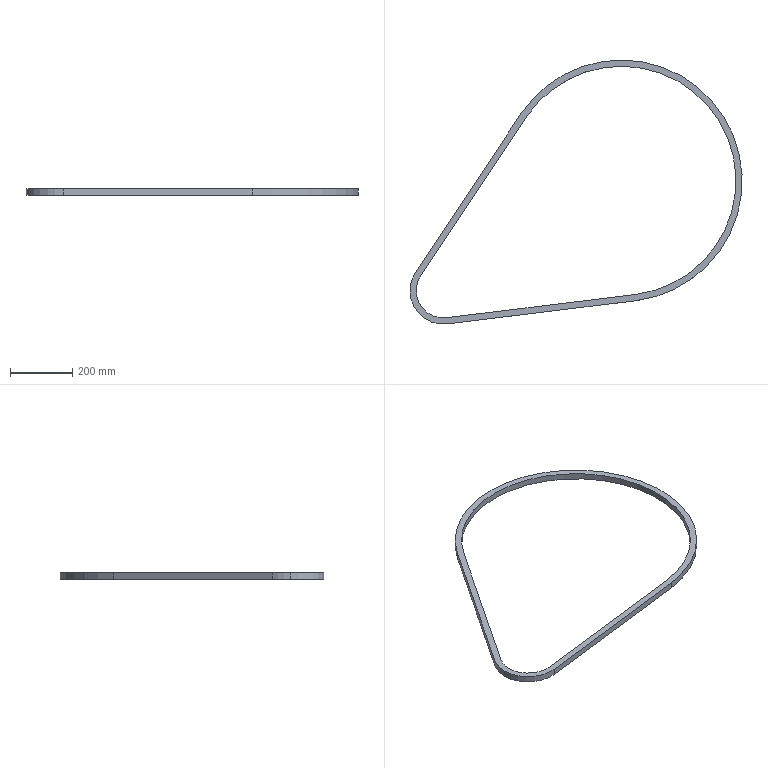Part | SolidWorks | features BaseBody 1 | 1 solid | 12 faces | box 1063 x 845.491 x 20 mm | volume 1178269 mm3 | cylinder 6 | plane 6 | commonest cylinder face diameters 173.589 x2 213.589 x2 733.102 x1 773.102 x1
STEP:
#1=CARTESIAN_POINT('',(-144.626,469.602,796.033));
#2=VERTEX_POINT('',#1);
#3=CARTESIAN_POINT('',(-513.842,1067.234,796.033));
#4=VERTEX_POINT('',#3);
#5=CARTESIAN_POINT('',(-191.923,853.249,796.033));
#6=DIRECTION('',(0.,0.,1.));
#7=DIRECTION('',(1.,0.,0.));
#8=AXIS2_PLACEMENT_3D('',#5,#6,#7);
#9=CIRCLE('',#8,386.551);
#10=EDGE_CURVE('',#2,#4,#9,.T.);
#11=ORIENTED_EDGE('',*,*,#10,.T.);
#12=CARTESIAN_POINT('',(-513.842,1067.234,816.033));
#13=VERTEX_POINT('',#12);
#14=CARTESIAN_POINT('',(-513.842,1067.234,816.033));
#15=DIRECTION('',(0.,0.,-1.));
#16=VECTOR('',#15,1000.);
#17=LINE('',#14,#16);
#18=EDGE_CURVE('',#13,#4,#17,.T.);
#19=ORIENTED_EDGE('',*,*,#18,.F.);
#20=CARTESIAN_POINT('',(-144.626,469.602,816.033));
#21=VERTEX_POINT('',#20);
#22=CARTESIAN_POINT('',(-191.923,853.249,816.033));
#23=DIRECTION('',(0.,0.,1.));
#24=DIRECTION('',(1.,0.,0.));
#25=AXIS2_PLACEMENT_3D('',#22,#23,#24);
#26=CIRCLE('',#25,386.551);
#27=EDGE_CURVE('',#21,#13,#26,.T.);
#28=ORIENTED_EDGE('',*,*,#27,.F.);
#29=CARTESIAN_POINT('',(-144.626,469.602,816.033));
#30=DIRECTION('',(0.,0.,-1.));
#31=VECTOR('',#30,1000.);
#32=LINE('',#29,#31);
#33=EDGE_CURVE('',#21,#2,#32,.T.);
#34=ORIENTED_EDGE('',*,*,#33,.T.);
#35=EDGE_LOOP('',(#11,#19,#28,#34));
#36=FACE_OUTER_BOUND('',#35,.T.);
#37=CARTESIAN_POINT('',(-191.923,853.249,816.033));
#38=DIRECTION('',(0.,0.,-1.));
#39=DIRECTION('',(-1.,0.,0.));
#40=AXIS2_PLACEMENT_3D('',#37,#38,#39);
#41=CYLINDRICAL_SURFACE('',#40,386.551);
#42=ADVANCED_FACE('',(#36),#41,.T.);
#43=CARTESIAN_POINT('',(-748.856,395.111,796.033));
#44=VERTEX_POINT('',#43);
#45=CARTESIAN_POINT('',(-748.856,395.111,796.033));
#46=DIRECTION('',(0.9925,0.1224,0.));
#47=VECTOR('',#46,1000.);
#48=LINE('',#45,#47);
#49=EDGE_CURVE('',#44,#2,#48,.T.);
#50=ORIENTED_EDGE('',*,*,#49,.T.);
#51=ORIENTED_EDGE('',*,*,#33,.F.);
#52=CARTESIAN_POINT('',(-748.856,395.111,816.033));
#53=VERTEX_POINT('',#52);
#54=CARTESIAN_POINT('',(-748.856,395.111,816.033));
#55=DIRECTION('',(0.9925,0.1224,0.));
#56=VECTOR('',#55,1000.);
#57=LINE('',#54,#56);
#58=EDGE_CURVE('',#53,#21,#57,.T.);
#59=ORIENTED_EDGE('',*,*,#58,.F.);
#60=CARTESIAN_POINT('',(-748.856,395.111,816.033));
#61=DIRECTION('',(0.,0.,-1.));
#62=VECTOR('',#61,1000.);
#63=LINE('',#60,#62);
#64=EDGE_CURVE('',#53,#44,#63,.T.);
#65=ORIENTED_EDGE('',*,*,#64,.T.);
#66=EDGE_LOOP('',(#50,#51,#59,#65));
#67=FACE_OUTER_BOUND('',#66,.T.);
#68=CARTESIAN_POINT('',(-748.856,395.111,816.033));
#69=DIRECTION('',(-0.1224,0.9925,0.));
#70=DIRECTION('',(0.,0.,1.));
#71=AXIS2_PLACEMENT_3D('',#68,#69,#70);
#72=PLANE('',#71);
#73=ADVANCED_FACE('',(#67),#72,.F.);
#74=CARTESIAN_POINT('',(-868.718,501.103,816.033));
#75=VERTEX_POINT('',#74);
#76=CARTESIAN_POINT('',(-868.718,501.103,796.033));
#77=VERTEX_POINT('',#76);
#78=CARTESIAN_POINT('',(-868.718,501.103,816.033));
#79=DIRECTION('',(0.,0.,-1.));
#80=VECTOR('',#79,1000.);
#81=LINE('',#78,#80);
#82=EDGE_CURVE('',#75,#77,#81,.T.);
#83=ORIENTED_EDGE('',*,*,#82,.F.);
#84=CARTESIAN_POINT('',(-850.862,560.222,816.033));
#85=VERTEX_POINT('',#84);
#86=CARTESIAN_POINT('',(-761.923,501.103,816.033));
#87=DIRECTION('',(0.,0.,1.));
#88=DIRECTION('',(1.,0.,0.));
#89=AXIS2_PLACEMENT_3D('',#86,#87,#88);
#90=CIRCLE('',#89,106.795);
#91=EDGE_CURVE('',#85,#75,#90,.T.);
#92=ORIENTED_EDGE('',*,*,#91,.F.);
#93=CARTESIAN_POINT('',(-850.862,560.222,796.033));
#94=VERTEX_POINT('',#93);
#95=CARTESIAN_POINT('',(-850.862,560.222,816.033));
#96=DIRECTION('',(0.,0.,-1.));
#97=VECTOR('',#96,1000.);
#98=LINE('',#95,#97);
#99=EDGE_CURVE('',#85,#94,#98,.T.);
#100=ORIENTED_EDGE('',*,*,#99,.T.);
#101=CARTESIAN_POINT('',(-761.923,501.103,796.033));
#102=DIRECTION('',(0.,0.,1.));
#103=DIRECTION('',(1.,0.,0.));
#104=AXIS2_PLACEMENT_3D('',#101,#102,#103);
#105=CIRCLE('',#104,106.795);
#106=EDGE_CURVE('',#94,#77,#105,.T.);
#107=ORIENTED_EDGE('',*,*,#106,.T.);
#108=EDGE_LOOP('',(#83,#92,#100,#107));
#109=FACE_OUTER_BOUND('',#108,.T.);
#110=CARTESIAN_POINT('',(-761.923,501.103,816.033));
#111=DIRECTION('',(0.,0.,-1.));
#112=DIRECTION('',(-1.,0.,0.));
#113=AXIS2_PLACEMENT_3D('',#110,#111,#112);
#114=CYLINDRICAL_SURFACE('',#113,106.795);
#115=ADVANCED_FACE('',(#109),#114,.T.);
#116=CARTESIAN_POINT('',(-513.842,1067.234,796.033));
#117=DIRECTION('',(-0.5536,-0.8328,0.));
#118=VECTOR('',#117,1000.);
#119=LINE('',#116,#118);
#120=EDGE_CURVE('',#4,#94,#119,.T.);
#121=ORIENTED_EDGE('',*,*,#120,.T.);
#122=ORIENTED_EDGE('',*,*,#99,.F.);
#123=CARTESIAN_POINT('',(-513.842,1067.234,816.033));
#124=DIRECTION('',(-0.5536,-0.8328,0.));
#125=VECTOR('',#124,1000.);
#126=LINE('',#123,#125);
#127=EDGE_CURVE('',#13,#85,#126,.T.);
#128=ORIENTED_EDGE('',*,*,#127,.F.);
#129=ORIENTED_EDGE('',*,*,#18,.T.);
#130=EDGE_LOOP('',(#121,#122,#128,#129));
#131=FACE_OUTER_BOUND('',#130,.T.);
#132=CARTESIAN_POINT('',(-513.842,1067.234,816.033));
#133=DIRECTION('',(0.8328,-0.5536,0.));
#134=DIRECTION('',(0.,0.,-1.));
#135=AXIS2_PLACEMENT_3D('',#132,#133,#134);
#136=PLANE('',#135);
#137=ADVANCED_FACE('',(#131),#136,.F.);
#138=CARTESIAN_POINT('',(-147.073,489.452,796.033));
#139=VERTEX_POINT('',#138);
#140=CARTESIAN_POINT('',(-497.186,1056.162,796.033));
#141=VERTEX_POINT('',#140);
#142=CARTESIAN_POINT('',(-191.923,853.249,796.033));
#143=DIRECTION('',(0.,0.,1.));
#144=DIRECTION('',(-1.,0.,0.));
#145=AXIS2_PLACEMENT_3D('',#142,#143,#144);
#146=CIRCLE('',#145,366.551);
#147=EDGE_CURVE('',#139,#141,#146,.T.);
#148=ORIENTED_EDGE('',*,*,#147,.F.);
#149=CARTESIAN_POINT('',(-147.073,489.452,816.033));
#150=VERTEX_POINT('',#149);
#151=CARTESIAN_POINT('',(-147.073,489.452,816.033));
#152=DIRECTION('',(0.,0.,-1.));
#153=VECTOR('',#152,1000.);
#154=LINE('',#151,#153);
#155=EDGE_CURVE('',#150,#139,#154,.T.);
#156=ORIENTED_EDGE('',*,*,#155,.F.);
#157=CARTESIAN_POINT('',(-497.186,1056.162,816.033));
#158=VERTEX_POINT('',#157);
#159=CARTESIAN_POINT('',(-191.923,853.249,816.033));
#160=DIRECTION('',(0.,0.,1.));
#161=DIRECTION('',(-1.,0.,0.));
#162=AXIS2_PLACEMENT_3D('',#159,#160,#161);
#163=CIRCLE('',#162,366.551);
#164=EDGE_CURVE('',#150,#158,#163,.T.);
#165=ORIENTED_EDGE('',*,*,#164,.T.);
#166=CARTESIAN_POINT('',(-497.186,1056.162,816.033));
#167=DIRECTION('',(0.,0.,-1.));
#168=VECTOR('',#167,1000.);
#169=LINE('',#166,#168);
#170=EDGE_CURVE('',#158,#141,#169,.T.);
#171=ORIENTED_EDGE('',*,*,#170,.T.);
#172=EDGE_LOOP('',(#148,#156,#165,#171));
#173=FACE_OUTER_BOUND('',#172,.T.);
#174=CARTESIAN_POINT('',(-191.923,853.249,816.033));
#175=DIRECTION('',(0.,0.,-1.));
#176=DIRECTION('',(-1.,0.,0.));
#177=AXIS2_PLACEMENT_3D('',#174,#175,#176);
#178=CYLINDRICAL_SURFACE('',#177,366.551);
#179=ADVANCED_FACE('',(#173),#178,.F.);
#180=CARTESIAN_POINT('',(-751.303,414.961,796.033));
#181=VERTEX_POINT('',#180);
#182=CARTESIAN_POINT('',(-751.303,414.961,796.033));
#183=DIRECTION('',(0.9925,0.1224,0.));
#184=VECTOR('',#183,1000.);
#185=LINE('',#182,#184);
#186=EDGE_CURVE('',#181,#139,#185,.T.);
#187=ORIENTED_EDGE('',*,*,#186,.F.);
#188=CARTESIAN_POINT('',(-751.303,414.961,816.033));
#189=VERTEX_POINT('',#188);
#190=CARTESIAN_POINT('',(-751.303,414.961,816.033));
#191=DIRECTION('',(0.,0.,-1.));
#192=VECTOR('',#191,1000.);
#193=LINE('',#190,#192);
#194=EDGE_CURVE('',#189,#181,#193,.T.);
#195=ORIENTED_EDGE('',*,*,#194,.F.);
#196=CARTESIAN_POINT('',(-751.303,414.961,816.033));
#197=DIRECTION('',(0.9925,0.1224,0.));
#198=VECTOR('',#197,1000.);
#199=LINE('',#196,#198);
#200=EDGE_CURVE('',#189,#150,#199,.T.);
#201=ORIENTED_EDGE('',*,*,#200,.T.);
#202=ORIENTED_EDGE('',*,*,#155,.T.);
#203=EDGE_LOOP('',(#187,#195,#201,#202));
#204=FACE_OUTER_BOUND('',#203,.T.);
#205=CARTESIAN_POINT('',(-751.303,414.961,816.033));
#206=DIRECTION('',(-0.1224,0.9925,0.));
#207=DIRECTION('',(0.,0.,1.));
#208=AXIS2_PLACEMENT_3D('',#205,#206,#207);
#209=PLANE('',#208);
#210=ADVANCED_FACE('',(#204),#209,.T.);
#211=CARTESIAN_POINT('',(-848.718,501.103,816.033));
#212=VERTEX_POINT('',#211);
#213=CARTESIAN_POINT('',(-848.718,501.103,796.033));
#214=VERTEX_POINT('',#213);
#215=CARTESIAN_POINT('',(-848.718,501.103,816.033));
#216=DIRECTION('',(0.,0.,-1.));
#217=VECTOR('',#216,1000.);
#218=LINE('',#215,#217);
#219=EDGE_CURVE('',#212,#214,#218,.T.);
#220=ORIENTED_EDGE('',*,*,#219,.F.);
#221=CARTESIAN_POINT('',(-761.923,501.103,816.033));
#222=DIRECTION('',(0.,0.,1.));
#223=DIRECTION('',(-1.,0.,0.));
#224=AXIS2_PLACEMENT_3D('',#221,#222,#223);
#225=CIRCLE('',#224,86.795);
#226=EDGE_CURVE('',#212,#189,#225,.T.);
#227=ORIENTED_EDGE('',*,*,#226,.T.);
#228=ORIENTED_EDGE('',*,*,#194,.T.);
#229=CARTESIAN_POINT('',(-761.923,501.103,796.033));
#230=DIRECTION('',(0.,0.,1.));
#231=DIRECTION('',(-1.,0.,0.));
#232=AXIS2_PLACEMENT_3D('',#229,#230,#231);
#233=CIRCLE('',#232,86.795);
#234=EDGE_CURVE('',#214,#181,#233,.T.);
#235=ORIENTED_EDGE('',*,*,#234,.F.);
#236=EDGE_LOOP('',(#220,#227,#228,#235));
#237=FACE_OUTER_BOUND('',#236,.T.);
#238=CARTESIAN_POINT('',(-761.923,501.103,816.033));
#239=DIRECTION('',(0.,0.,-1.));
#240=DIRECTION('',(-1.,0.,0.));
#241=AXIS2_PLACEMENT_3D('',#238,#239,#240);
#242=CYLINDRICAL_SURFACE('',#241,86.795);
#243=ADVANCED_FACE('',(#237),#242,.F.);
#244=CARTESIAN_POINT('',(-834.206,549.151,796.033));
#245=VERTEX_POINT('',#244);
#246=CARTESIAN_POINT('',(-497.186,1056.162,796.033));
#247=DIRECTION('',(-0.5536,-0.8328,0.));
#248=VECTOR('',#247,1000.);
#249=LINE('',#246,#248);
#250=EDGE_CURVE('',#141,#245,#249,.T.);
#251=ORIENTED_EDGE('',*,*,#250,.F.);
#252=ORIENTED_EDGE('',*,*,#170,.F.);
#253=CARTESIAN_POINT('',(-834.206,549.151,816.033));
#254=VERTEX_POINT('',#253);
#255=CARTESIAN_POINT('',(-497.186,1056.162,816.033));
#256=DIRECTION('',(-0.5536,-0.8328,0.));
#257=VECTOR('',#256,1000.);
#258=LINE('',#255,#257);
#259=EDGE_CURVE('',#158,#254,#258,.T.);
#260=ORIENTED_EDGE('',*,*,#259,.T.);
#261=CARTESIAN_POINT('',(-834.206,549.151,816.033));
#262=DIRECTION('',(0.,0.,-1.));
#263=VECTOR('',#262,1000.);
#264=LINE('',#261,#263);
#265=EDGE_CURVE('',#254,#245,#264,.T.);
#266=ORIENTED_EDGE('',*,*,#265,.T.);
#267=EDGE_LOOP('',(#251,#252,#260,#266));
#268=FACE_OUTER_BOUND('',#267,.T.);
#269=CARTESIAN_POINT('',(-497.186,1056.162,816.033));
#270=DIRECTION('',(0.8328,-0.5536,0.));
#271=DIRECTION('',(0.,0.,-1.));
#272=AXIS2_PLACEMENT_3D('',#269,#270,#271);
#273=PLANE('',#272);
#274=ADVANCED_FACE('',(#268),#273,.T.);
#275=ORIENTED_EDGE('',*,*,#259,.F.);
#276=ORIENTED_EDGE('',*,*,#164,.F.);
#277=ORIENTED_EDGE('',*,*,#200,.F.);
#278=ORIENTED_EDGE('',*,*,#226,.F.);
#279=CARTESIAN_POINT('',(-761.923,501.103,816.033));
#280=DIRECTION('',(0.,0.,1.));
#281=DIRECTION('',(-1.,0.,0.));
#282=AXIS2_PLACEMENT_3D('',#279,#280,#281);
#283=CIRCLE('',#282,86.795);
#284=EDGE_CURVE('',#254,#212,#283,.T.);
#285=ORIENTED_EDGE('',*,*,#284,.F.);
#286=EDGE_LOOP('',(#275,#276,#277,#278,#285));
#287=FACE_BOUND('',#286,.T.);
#288=ORIENTED_EDGE('',*,*,#27,.T.);
#289=ORIENTED_EDGE('',*,*,#127,.T.);
#290=ORIENTED_EDGE('',*,*,#91,.T.);
#291=CARTESIAN_POINT('',(-761.923,501.103,816.033));
#292=DIRECTION('',(0.,0.,1.));
#293=DIRECTION('',(1.,0.,0.));
#294=AXIS2_PLACEMENT_3D('',#291,#292,#293);
#295=CIRCLE('',#294,106.795);
#296=EDGE_CURVE('',#75,#53,#295,.T.);
#297=ORIENTED_EDGE('',*,*,#296,.T.);
#298=ORIENTED_EDGE('',*,*,#58,.T.);
#299=EDGE_LOOP('',(#288,#289,#290,#297,#298));
#300=FACE_OUTER_BOUND('',#299,.T.);
#301=CARTESIAN_POINT('',(-191.923,853.249,816.033));
#302=DIRECTION('',(0.,0.,-1.));
#303=DIRECTION('',(0.,-1.,0.));
#304=AXIS2_PLACEMENT_3D('',#301,#302,#303);
#305=PLANE('',#304);
#306=ADVANCED_FACE('',(#287,#300),#305,.F.);
#307=ORIENTED_EDGE('',*,*,#250,.T.);
#308=CARTESIAN_POINT('',(-761.923,501.103,796.033));
#309=DIRECTION('',(0.,0.,1.));
#310=DIRECTION('',(-1.,0.,0.));
#311=AXIS2_PLACEMENT_3D('',#308,#309,#310);
#312=CIRCLE('',#311,86.795);
#313=EDGE_CURVE('',#245,#214,#312,.T.);
#314=ORIENTED_EDGE('',*,*,#313,.T.);
#315=ORIENTED_EDGE('',*,*,#234,.T.);
#316=ORIENTED_EDGE('',*,*,#186,.T.);
#317=ORIENTED_EDGE('',*,*,#147,.T.);
#318=EDGE_LOOP('',(#307,#314,#315,#316,#317));
#319=FACE_BOUND('',#318,.T.);
#320=ORIENTED_EDGE('',*,*,#106,.F.);
#321=ORIENTED_EDGE('',*,*,#120,.F.);
#322=ORIENTED_EDGE('',*,*,#10,.F.);
#323=ORIENTED_EDGE('',*,*,#49,.F.);
#324=CARTESIAN_POINT('',(-761.923,501.103,796.033));
#325=DIRECTION('',(0.,0.,1.));
#326=DIRECTION('',(1.,0.,0.));
#327=AXIS2_PLACEMENT_3D('',#324,#325,#326);
#328=CIRCLE('',#327,106.795);
#329=EDGE_CURVE('',#77,#44,#328,.T.);
#330=ORIENTED_EDGE('',*,*,#329,.F.);
#331=EDGE_LOOP('',(#320,#321,#322,#323,#330));
#332=FACE_OUTER_BOUND('',#331,.T.);
#333=CARTESIAN_POINT('',(-761.923,501.103,796.033));
#334=DIRECTION('',(0.,0.,-1.));
#335=DIRECTION('',(0.,-1.,0.));
#336=AXIS2_PLACEMENT_3D('',#333,#334,#335);
#337=PLANE('',#336);
#338=ADVANCED_FACE('',(#319,#332),#337,.T.);
#339=ORIENTED_EDGE('',*,*,#284,.T.);
#340=ORIENTED_EDGE('',*,*,#219,.T.);
#341=ORIENTED_EDGE('',*,*,#313,.F.);
#342=ORIENTED_EDGE('',*,*,#265,.F.);
#343=EDGE_LOOP('',(#339,#340,#341,#342));
#344=FACE_OUTER_BOUND('',#343,.T.);
#345=CARTESIAN_POINT('',(-761.923,501.103,816.033));
#346=DIRECTION('',(0.,0.,-1.));
#347=DIRECTION('',(-1.,0.,0.));
#348=AXIS2_PLACEMENT_3D('',#345,#346,#347);
#349=CYLINDRICAL_SURFACE('',#348,86.795);
#350=ADVANCED_FACE('',(#344),#349,.F.);
#351=ORIENTED_EDGE('',*,*,#296,.F.);
#352=ORIENTED_EDGE('',*,*,#82,.T.);
#353=ORIENTED_EDGE('',*,*,#329,.T.);
#354=ORIENTED_EDGE('',*,*,#64,.F.);
#355=EDGE_LOOP('',(#351,#352,#353,#354));
#356=FACE_OUTER_BOUND('',#355,.T.);
#357=CARTESIAN_POINT('',(-761.923,501.103,816.033));
#358=DIRECTION('',(0.,0.,-1.));
#359=DIRECTION('',(-1.,0.,0.));
#360=AXIS2_PLACEMENT_3D('',#357,#358,#359);
#361=CYLINDRICAL_SURFACE('',#360,106.795);
#362=ADVANCED_FACE('',(#356),#361,.T.);
#363=CLOSED_SHELL('',(#42,#73,#115,#137,#179,#210,#243,#274,#306,#338,#350,#362));
#364=MANIFOLD_SOLID_BREP('',#363);
#365=CARTESIAN_POINT('',(0.,0.,0.));
#366=DIRECTION('',(0.,0.,1.));
#367=DIRECTION('',(1.,0.,0.));
#368=AXIS2_PLACEMENT_3D('',#365,#366,#367);
#369=(LENGTH_UNIT()NAMED_UNIT(*)SI_UNIT(.MILLI.,.METRE.));
#370=UNCERTAINTY_MEASURE_WITH_UNIT(LENGTH_MEASURE(0.00001),#369,'','');
#371=(NAMED_UNIT(*)PLANE_ANGLE_UNIT()SI_UNIT($,.RADIAN.));
#372=(NAMED_UNIT(*)SI_UNIT($,.STERADIAN.)SOLID_ANGLE_UNIT());
#373=(GEOMETRIC_REPRESENTATION_CONTEXT(3)GLOBAL_UNCERTAINTY_ASSIGNED_CONTEXT((#370))GLOBAL_UNIT_ASSIGNED_CONTEXT((#369,#371,#372))REPRESENTATION_CONTEXT('',''));
#374=ADVANCED_BREP_SHAPE_REPRESENTATION('',(#364,#368),#373);